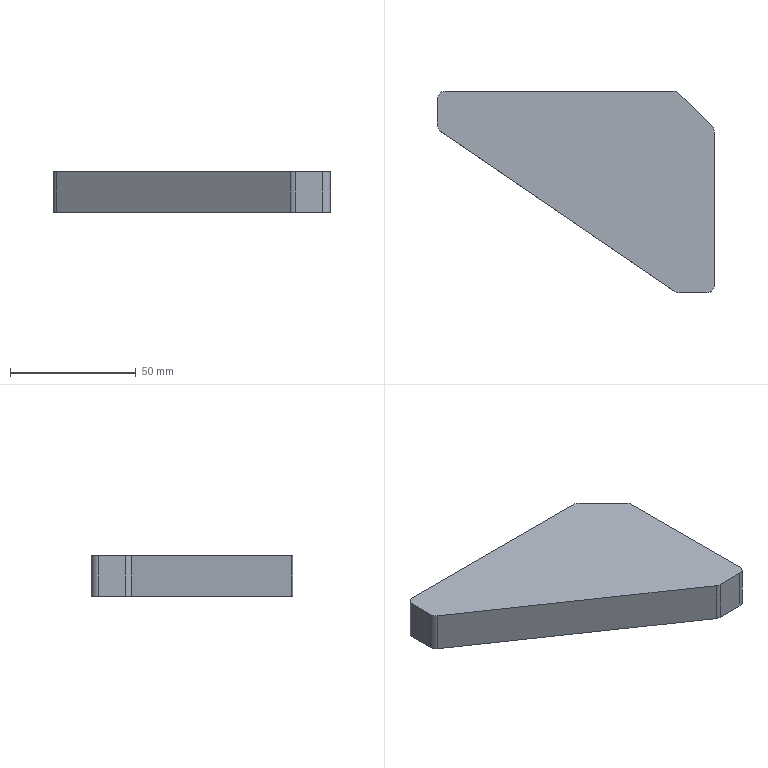Part | STEP file | Copy (1) of SN10_008_007-03_REFORCO | 1 solid | 14 faces | box 110 x 80 x 16 mm | volume 89525 mm3 | plane 8 | cylinder 6 | commonest cylinder face diameters 6 x6
STEP:
#1=CARTESIAN_POINT('',(0.,0.,0.));
#2=DIRECTION('',(0.,0.,1.));
#3=DIRECTION('',(1.,0.,0.));
#4=AXIS2_PLACEMENT_3D('',#1,#2,#3);
#5=CARTESIAN_POINT('',(243.629,237.,420.27));
#6=VERTEX_POINT('',#5);
#7=CARTESIAN_POINT('',(246.629,240.,420.27));
#8=VERTEX_POINT('',#7);
#9=CARTESIAN_POINT('',(246.629,237.,420.27));
#10=DIRECTION('',(0.,0.,-1.));
#11=DIRECTION('',(1.,0.,0.));
#12=AXIS2_PLACEMENT_3D('',#9,#10,#11);
#13=CIRCLE('',#12,3.);
#14=CARTESIAN_POINT('',(246.629,237.,428.27));
#15=DIRECTION('',(0.,0.,-1.));
#16=DIRECTION('',(-1.,0.,0.));
#17=AXIS2_PLACEMENT_3D('',#14,#15,#16);
#18=CYLINDRICAL_SURFACE('',#17,3.);
#19=CARTESIAN_POINT('',(-3.142,8.));
#20=DIRECTION('',(1.,0.));
#21=VECTOR('',#20,1.);
#22=LINE('',#19,#21);
#23=(GEOMETRIC_REPRESENTATION_CONTEXT(2)PARAMETRIC_REPRESENTATION_CONTEXT()REPRESENTATION_CONTEXT('',''));
#24=DEFINITIONAL_REPRESENTATION('',(#22),#23);
#25=PCURVE('',#18,#24);
#26=CARTESIAN_POINT('',(0.,0.,420.27));
#27=DIRECTION('',(0.,0.,-1.));
#28=DIRECTION('',(-1.,0.,0.));
#29=AXIS2_PLACEMENT_3D('',#26,#27,#28);
#30=PLANE('',#29);
#31=CARTESIAN_POINT('',(-246.629,237.));
#32=DIRECTION('',(-1.,0.));
#33=AXIS2_PLACEMENT_2D('',#31,#32);
#34=CIRCLE('',#33,3.);
#35=(GEOMETRIC_REPRESENTATION_CONTEXT(2)PARAMETRIC_REPRESENTATION_CONTEXT()REPRESENTATION_CONTEXT('',''));
#36=DEFINITIONAL_REPRESENTATION('',(#34),#35);
#37=PCURVE('',#30,#36);
#38=SURFACE_CURVE('',#13,(#25,#37),.PCURVE_S1.);
#39=EDGE_CURVE('',#6,#8,#38,.T.);
#40=ORIENTED_EDGE('',*,*,#39,.F.);
#41=CARTESIAN_POINT('',(243.629,237.,436.27));
#42=VERTEX_POINT('',#41);
#43=CARTESIAN_POINT('',(243.629,237.,436.27));
#44=DIRECTION('',(0.,0.,-1.));
#45=VECTOR('',#44,1.);
#46=LINE('',#43,#45);
#47=CARTESIAN_POINT('',(0.,-8.));
#48=DIRECTION('',(0.,1.));
#49=VECTOR('',#48,1.);
#50=LINE('',#47,#49);
#51=(GEOMETRIC_REPRESENTATION_CONTEXT(2)PARAMETRIC_REPRESENTATION_CONTEXT()REPRESENTATION_CONTEXT('',''));
#52=DEFINITIONAL_REPRESENTATION('',(#50),#51);
#53=PCURVE('',#18,#52);
#54=CARTESIAN_POINT('',(243.629,225.,436.27));
#55=DIRECTION('',(-1.,0.,0.));
#56=DIRECTION('',(0.,0.,1.));
#57=AXIS2_PLACEMENT_3D('',#54,#55,#56);
#58=PLANE('',#57);
#59=CARTESIAN_POINT('',(0.,12.));
#60=DIRECTION('',(-1.,0.));
#61=VECTOR('',#60,1.);
#62=LINE('',#59,#61);
#63=(GEOMETRIC_REPRESENTATION_CONTEXT(2)PARAMETRIC_REPRESENTATION_CONTEXT()REPRESENTATION_CONTEXT('',''));
#64=DEFINITIONAL_REPRESENTATION('',(#62),#63);
#65=PCURVE('',#58,#64);
#66=SURFACE_CURVE('',#46,(#53,#65),.PCURVE_S1.);
#67=EDGE_CURVE('',#42,#6,#66,.T.);
#68=ORIENTED_EDGE('',*,*,#67,.F.);
#69=CARTESIAN_POINT('',(246.629,240.,436.27));
#70=VERTEX_POINT('',#69);
#71=CARTESIAN_POINT('',(246.629,237.,436.27));
#72=DIRECTION('',(0.,0.,-1.));
#73=DIRECTION('',(1.,0.,0.));
#74=AXIS2_PLACEMENT_3D('',#71,#72,#73);
#75=CIRCLE('',#74,3.);
#76=CARTESIAN_POINT('',(-3.142,-8.));
#77=DIRECTION('',(1.,0.));
#78=VECTOR('',#77,1.);
#79=LINE('',#76,#78);
#80=(GEOMETRIC_REPRESENTATION_CONTEXT(2)PARAMETRIC_REPRESENTATION_CONTEXT()REPRESENTATION_CONTEXT('',''));
#81=DEFINITIONAL_REPRESENTATION('',(#79),#80);
#82=PCURVE('',#18,#81);
#83=CARTESIAN_POINT('',(0.,0.,436.27));
#84=DIRECTION('',(0.,0.,-1.));
#85=DIRECTION('',(-1.,0.,0.));
#86=AXIS2_PLACEMENT_3D('',#83,#84,#85);
#87=PLANE('',#86);
#88=CARTESIAN_POINT('',(-246.629,237.));
#89=DIRECTION('',(-1.,0.));
#90=AXIS2_PLACEMENT_2D('',#88,#89);
#91=CIRCLE('',#90,3.);
#92=(GEOMETRIC_REPRESENTATION_CONTEXT(2)PARAMETRIC_REPRESENTATION_CONTEXT()REPRESENTATION_CONTEXT('',''));
#93=DEFINITIONAL_REPRESENTATION('',(#91),#92);
#94=PCURVE('',#87,#93);
#95=SURFACE_CURVE('',#75,(#82,#94),.PCURVE_S1.);
#96=EDGE_CURVE('',#42,#70,#95,.T.);
#97=ORIENTED_EDGE('',*,*,#96,.T.);
#98=CARTESIAN_POINT('',(246.629,240.,436.27));
#99=DIRECTION('',(0.,0.,-1.));
#100=VECTOR('',#99,1.);
#101=LINE('',#98,#100);
#102=CARTESIAN_POINT('',(1.571,-8.));
#103=DIRECTION('',(0.,1.));
#104=VECTOR('',#103,1.);
#105=LINE('',#102,#104);
#106=(GEOMETRIC_REPRESENTATION_CONTEXT(2)PARAMETRIC_REPRESENTATION_CONTEXT()REPRESENTATION_CONTEXT('',''));
#107=DEFINITIONAL_REPRESENTATION('',(#105),#106);
#108=PCURVE('',#18,#107);
#109=CARTESIAN_POINT('',(243.629,240.,436.27));
#110=DIRECTION('',(0.,1.,0.));
#111=DIRECTION('',(0.,0.,1.));
#112=AXIS2_PLACEMENT_3D('',#109,#110,#111);
#113=PLANE('',#112);
#114=CARTESIAN_POINT('',(0.,3.));
#115=DIRECTION('',(-1.,0.));
#116=VECTOR('',#115,1.);
#117=LINE('',#114,#116);
#118=(GEOMETRIC_REPRESENTATION_CONTEXT(2)PARAMETRIC_REPRESENTATION_CONTEXT()REPRESENTATION_CONTEXT('',''));
#119=DEFINITIONAL_REPRESENTATION('',(#117),#118);
#120=PCURVE('',#113,#119);
#121=SURFACE_CURVE('',#101,(#108,#120),.PCURVE_S1.);
#122=EDGE_CURVE('',#70,#8,#121,.T.);
#123=ORIENTED_EDGE('',*,*,#122,.T.);
#124=EDGE_LOOP('',(#40,#68,#97,#123));
#125=FACE_BOUND('',#124,.T.);
#126=ADVANCED_FACE('',(#125),#18,.T.);
#127=CARTESIAN_POINT('',(243.629,226.582,436.27));
#128=VERTEX_POINT('',#127);
#129=CARTESIAN_POINT('',(243.629,226.582,436.27));
#130=DIRECTION('',(0.,1.,0.));
#131=VECTOR('',#130,1.);
#132=LINE('',#129,#131);
#133=CARTESIAN_POINT('',(0.,1.582));
#134=DIRECTION('',(0.,1.));
#135=VECTOR('',#134,1.);
#136=LINE('',#133,#135);
#137=(GEOMETRIC_REPRESENTATION_CONTEXT(2)PARAMETRIC_REPRESENTATION_CONTEXT()REPRESENTATION_CONTEXT('',''));
#138=DEFINITIONAL_REPRESENTATION('',(#136),#137);
#139=PCURVE('',#58,#138);
#140=CARTESIAN_POINT('',(-243.629,226.582));
#141=DIRECTION('',(0.,1.));
#142=VECTOR('',#141,1.);
#143=LINE('',#140,#142);
#144=(GEOMETRIC_REPRESENTATION_CONTEXT(2)PARAMETRIC_REPRESENTATION_CONTEXT()REPRESENTATION_CONTEXT('',''));
#145=DEFINITIONAL_REPRESENTATION('',(#143),#144);
#146=PCURVE('',#87,#145);
#147=SURFACE_CURVE('',#132,(#139,#146),.PCURVE_S1.);
#148=EDGE_CURVE('',#128,#42,#147,.T.);
#149=ORIENTED_EDGE('',*,*,#148,.T.);
#150=ORIENTED_EDGE('',*,*,#67,.T.);
#151=CARTESIAN_POINT('',(243.629,226.582,420.27));
#152=VERTEX_POINT('',#151);
#153=CARTESIAN_POINT('',(243.629,226.582,420.27));
#154=DIRECTION('',(0.,1.,0.));
#155=VECTOR('',#154,1.);
#156=LINE('',#153,#155);
#157=CARTESIAN_POINT('',(-16.,1.582));
#158=DIRECTION('',(0.,1.));
#159=VECTOR('',#158,1.);
#160=LINE('',#157,#159);
#161=(GEOMETRIC_REPRESENTATION_CONTEXT(2)PARAMETRIC_REPRESENTATION_CONTEXT()REPRESENTATION_CONTEXT('',''));
#162=DEFINITIONAL_REPRESENTATION('',(#160),#161);
#163=PCURVE('',#58,#162);
#164=CARTESIAN_POINT('',(-243.629,226.582));
#165=DIRECTION('',(0.,1.));
#166=VECTOR('',#165,1.);
#167=LINE('',#164,#166);
#168=(GEOMETRIC_REPRESENTATION_CONTEXT(2)PARAMETRIC_REPRESENTATION_CONTEXT()REPRESENTATION_CONTEXT('',''));
#169=DEFINITIONAL_REPRESENTATION('',(#167),#168);
#170=PCURVE('',#30,#169);
#171=SURFACE_CURVE('',#156,(#163,#170),.PCURVE_S1.);
#172=EDGE_CURVE('',#152,#6,#171,.T.);
#173=ORIENTED_EDGE('',*,*,#172,.F.);
#174=CARTESIAN_POINT('',(243.629,226.582,436.27));
#175=DIRECTION('',(0.,0.,-1.));
#176=VECTOR('',#175,1.);
#177=LINE('',#174,#176);
#178=CARTESIAN_POINT('',(0.,1.582));
#179=DIRECTION('',(-1.,0.));
#180=VECTOR('',#179,1.);
#181=LINE('',#178,#180);
#182=(GEOMETRIC_REPRESENTATION_CONTEXT(2)PARAMETRIC_REPRESENTATION_CONTEXT()REPRESENTATION_CONTEXT('',''));
#183=DEFINITIONAL_REPRESENTATION('',(#181),#182);
#184=PCURVE('',#58,#183);
#185=CARTESIAN_POINT('',(246.629,226.582,428.27));
#186=DIRECTION('',(0.,0.,-1.));
#187=DIRECTION('',(-0.5647,-0.8253,0.));
#188=AXIS2_PLACEMENT_3D('',#185,#186,#187);
#189=CYLINDRICAL_SURFACE('',#188,3.);
#190=CARTESIAN_POINT('',(0.9707,-8.));
#191=DIRECTION('',(0.,1.));
#192=VECTOR('',#191,1.);
#193=LINE('',#190,#192);
#194=(GEOMETRIC_REPRESENTATION_CONTEXT(2)PARAMETRIC_REPRESENTATION_CONTEXT()REPRESENTATION_CONTEXT('',''));
#195=DEFINITIONAL_REPRESENTATION('',(#193),#194);
#196=PCURVE('',#189,#195);
#197=SURFACE_CURVE('',#177,(#184,#196),.PCURVE_S1.);
#198=EDGE_CURVE('',#128,#152,#197,.T.);
#199=ORIENTED_EDGE('',*,*,#198,.F.);
#200=EDGE_LOOP('',(#149,#150,#173,#199));
#201=FACE_BOUND('',#200,.T.);
#202=ADVANCED_FACE('',(#201),#58,.T.);
#203=CARTESIAN_POINT('',(244.935,224.106,420.27));
#204=VERTEX_POINT('',#203);
#205=CARTESIAN_POINT('',(246.629,226.582,420.27));
#206=DIRECTION('',(0.,0.,-1.));
#207=DIRECTION('',(1.,0.,0.));
#208=AXIS2_PLACEMENT_3D('',#205,#206,#207);
#209=CIRCLE('',#208,3.);
#210=CARTESIAN_POINT('',(-2.171,8.));
#211=DIRECTION('',(1.,0.));
#212=VECTOR('',#211,1.);
#213=LINE('',#210,#212);
#214=(GEOMETRIC_REPRESENTATION_CONTEXT(2)PARAMETRIC_REPRESENTATION_CONTEXT()REPRESENTATION_CONTEXT('',''));
#215=DEFINITIONAL_REPRESENTATION('',(#213),#214);
#216=PCURVE('',#189,#215);
#217=CARTESIAN_POINT('',(-246.629,226.582));
#218=DIRECTION('',(-1.,0.));
#219=AXIS2_PLACEMENT_2D('',#217,#218);
#220=CIRCLE('',#219,3.);
#221=(GEOMETRIC_REPRESENTATION_CONTEXT(2)PARAMETRIC_REPRESENTATION_CONTEXT()REPRESENTATION_CONTEXT('',''));
#222=DEFINITIONAL_REPRESENTATION('',(#220),#221);
#223=PCURVE('',#30,#222);
#224=SURFACE_CURVE('',#209,(#216,#223),.PCURVE_S1.);
#225=EDGE_CURVE('',#204,#152,#224,.T.);
#226=ORIENTED_EDGE('',*,*,#225,.F.);
#227=CARTESIAN_POINT('',(244.935,224.106,436.27));
#228=VERTEX_POINT('',#227);
#229=CARTESIAN_POINT('',(244.935,224.106,436.27));
#230=DIRECTION('',(0.,0.,-1.));
#231=VECTOR('',#230,1.);
#232=LINE('',#229,#231);
#233=CARTESIAN_POINT('',(0.,-8.));
#234=DIRECTION('',(0.,1.));
#235=VECTOR('',#234,1.);
#236=LINE('',#233,#235);
#237=(GEOMETRIC_REPRESENTATION_CONTEXT(2)PARAMETRIC_REPRESENTATION_CONTEXT()REPRESENTATION_CONTEXT('',''));
#238=DEFINITIONAL_REPRESENTATION('',(#236),#237);
#239=PCURVE('',#189,#238);
#240=CARTESIAN_POINT('',(338.629,160.,436.27));
#241=DIRECTION('',(-0.5647,-0.8253,0.));
#242=DIRECTION('',(0.,0.,1.));
#243=AXIS2_PLACEMENT_3D('',#240,#241,#242);
#244=PLANE('',#243);
#245=CARTESIAN_POINT('',(0.,113.526));
#246=DIRECTION('',(-1.,0.));
#247=VECTOR('',#246,1.);
#248=LINE('',#245,#247);
#249=(GEOMETRIC_REPRESENTATION_CONTEXT(2)PARAMETRIC_REPRESENTATION_CONTEXT()REPRESENTATION_CONTEXT('',''));
#250=DEFINITIONAL_REPRESENTATION('',(#248),#249);
#251=PCURVE('',#244,#250);
#252=SURFACE_CURVE('',#232,(#239,#251),.PCURVE_S1.);
#253=EDGE_CURVE('',#228,#204,#252,.T.);
#254=ORIENTED_EDGE('',*,*,#253,.F.);
#255=CARTESIAN_POINT('',(246.629,226.582,436.27));
#256=DIRECTION('',(0.,0.,-1.));
#257=DIRECTION('',(1.,0.,0.));
#258=AXIS2_PLACEMENT_3D('',#255,#256,#257);
#259=CIRCLE('',#258,3.);
#260=CARTESIAN_POINT('',(-2.171,-8.));
#261=DIRECTION('',(1.,0.));
#262=VECTOR('',#261,1.);
#263=LINE('',#260,#262);
#264=(GEOMETRIC_REPRESENTATION_CONTEXT(2)PARAMETRIC_REPRESENTATION_CONTEXT()REPRESENTATION_CONTEXT('',''));
#265=DEFINITIONAL_REPRESENTATION('',(#263),#264);
#266=PCURVE('',#189,#265);
#267=CARTESIAN_POINT('',(-246.629,226.582));
#268=DIRECTION('',(-1.,0.));
#269=AXIS2_PLACEMENT_2D('',#267,#268);
#270=CIRCLE('',#269,3.);
#271=(GEOMETRIC_REPRESENTATION_CONTEXT(2)PARAMETRIC_REPRESENTATION_CONTEXT()REPRESENTATION_CONTEXT('',''));
#272=DEFINITIONAL_REPRESENTATION('',(#270),#271);
#273=PCURVE('',#87,#272);
#274=SURFACE_CURVE('',#259,(#266,#273),.PCURVE_S1.);
#275=EDGE_CURVE('',#228,#128,#274,.T.);
#276=ORIENTED_EDGE('',*,*,#275,.T.);
#277=ORIENTED_EDGE('',*,*,#198,.T.);
#278=EDGE_LOOP('',(#226,#254,#276,#277));
#279=FACE_BOUND('',#278,.T.);
#280=ADVANCED_FACE('',(#279),#189,.T.);
#281=CARTESIAN_POINT('',(337.863,160.524,436.27));
#282=VERTEX_POINT('',#281);
#283=CARTESIAN_POINT('',(337.863,160.524,436.27));
#284=DIRECTION('',(-0.8253,0.5647,0.));
#285=VECTOR('',#284,1.);
#286=LINE('',#283,#285);
#287=CARTESIAN_POINT('',(0.,0.9281));
#288=DIRECTION('',(0.,1.));
#289=VECTOR('',#288,1.);
#290=LINE('',#287,#289);
#291=(GEOMETRIC_REPRESENTATION_CONTEXT(2)PARAMETRIC_REPRESENTATION_CONTEXT()REPRESENTATION_CONTEXT('',''));
#292=DEFINITIONAL_REPRESENTATION('',(#290),#291);
#293=PCURVE('',#244,#292);
#294=CARTESIAN_POINT('',(-337.863,160.524));
#295=DIRECTION('',(0.8253,0.5647));
#296=VECTOR('',#295,1.);
#297=LINE('',#294,#296);
#298=(GEOMETRIC_REPRESENTATION_CONTEXT(2)PARAMETRIC_REPRESENTATION_CONTEXT()REPRESENTATION_CONTEXT('',''));
#299=DEFINITIONAL_REPRESENTATION('',(#297),#298);
#300=PCURVE('',#87,#299);
#301=SURFACE_CURVE('',#286,(#293,#300),.PCURVE_S1.);
#302=EDGE_CURVE('',#282,#228,#301,.T.);
#303=ORIENTED_EDGE('',*,*,#302,.T.);
#304=ORIENTED_EDGE('',*,*,#253,.T.);
#305=CARTESIAN_POINT('',(337.863,160.524,420.27));
#306=VERTEX_POINT('',#305);
#307=CARTESIAN_POINT('',(337.863,160.524,420.27));
#308=DIRECTION('',(-0.8253,0.5647,0.));
#309=VECTOR('',#308,1.);
#310=LINE('',#307,#309);
#311=CARTESIAN_POINT('',(-16.,0.9281));
#312=DIRECTION('',(0.,1.));
#313=VECTOR('',#312,1.);
#314=LINE('',#311,#313);
#315=(GEOMETRIC_REPRESENTATION_CONTEXT(2)PARAMETRIC_REPRESENTATION_CONTEXT()REPRESENTATION_CONTEXT('',''));
#316=DEFINITIONAL_REPRESENTATION('',(#314),#315);
#317=PCURVE('',#244,#316);
#318=CARTESIAN_POINT('',(-337.863,160.524));
#319=DIRECTION('',(0.8253,0.5647));
#320=VECTOR('',#319,1.);
#321=LINE('',#318,#320);
#322=(GEOMETRIC_REPRESENTATION_CONTEXT(2)PARAMETRIC_REPRESENTATION_CONTEXT()REPRESENTATION_CONTEXT('',''));
#323=DEFINITIONAL_REPRESENTATION('',(#321),#322);
#324=PCURVE('',#30,#323);
#325=SURFACE_CURVE('',#310,(#317,#324),.PCURVE_S1.);
#326=EDGE_CURVE('',#306,#204,#325,.T.);
#327=ORIENTED_EDGE('',*,*,#326,.F.);
#328=CARTESIAN_POINT('',(337.863,160.524,436.27));
#329=DIRECTION('',(0.,0.,-1.));
#330=VECTOR('',#329,1.);
#331=LINE('',#328,#330);
#332=CARTESIAN_POINT('',(0.,0.9281));
#333=DIRECTION('',(-1.,0.));
#334=VECTOR('',#333,1.);
#335=LINE('',#332,#334);
#336=(GEOMETRIC_REPRESENTATION_CONTEXT(2)PARAMETRIC_REPRESENTATION_CONTEXT()REPRESENTATION_CONTEXT('',''));
#337=DEFINITIONAL_REPRESENTATION('',(#335),#336);
#338=PCURVE('',#244,#337);
#339=CARTESIAN_POINT('',(339.557,163.,428.27));
#340=DIRECTION('',(0.,0.,-1.));
#341=DIRECTION('',(0.,-1.,0.));
#342=AXIS2_PLACEMENT_3D('',#339,#340,#341);
#343=CYLINDRICAL_SURFACE('',#342,3.);
#344=CARTESIAN_POINT('',(0.6001,-8.));
#345=DIRECTION('',(0.,1.));
#346=VECTOR('',#345,1.);
#347=LINE('',#344,#346);
#348=(GEOMETRIC_REPRESENTATION_CONTEXT(2)PARAMETRIC_REPRESENTATION_CONTEXT()REPRESENTATION_CONTEXT('',''));
#349=DEFINITIONAL_REPRESENTATION('',(#347),#348);
#350=PCURVE('',#343,#349);
#351=SURFACE_CURVE('',#331,(#338,#350),.PCURVE_S1.);
#352=EDGE_CURVE('',#282,#306,#351,.T.);
#353=ORIENTED_EDGE('',*,*,#352,.F.);
#354=EDGE_LOOP('',(#303,#304,#327,#353));
#355=FACE_BOUND('',#354,.T.);
#356=ADVANCED_FACE('',(#355),#244,.T.);
#357=CARTESIAN_POINT('',(339.557,160.,420.27));
#358=VERTEX_POINT('',#357);
#359=CARTESIAN_POINT('',(339.557,163.,420.27));
#360=DIRECTION('',(0.,0.,-1.));
#361=DIRECTION('',(1.,0.,0.));
#362=AXIS2_PLACEMENT_3D('',#359,#360,#361);
#363=CIRCLE('',#362,3.);
#364=CARTESIAN_POINT('',(-1.571,8.));
#365=DIRECTION('',(1.,0.));
#366=VECTOR('',#365,1.);
#367=LINE('',#364,#366);
#368=(GEOMETRIC_REPRESENTATION_CONTEXT(2)PARAMETRIC_REPRESENTATION_CONTEXT()REPRESENTATION_CONTEXT('',''));
#369=DEFINITIONAL_REPRESENTATION('',(#367),#368);
#370=PCURVE('',#343,#369);
#371=CARTESIAN_POINT('',(-339.557,163.));
#372=DIRECTION('',(-1.,0.));
#373=AXIS2_PLACEMENT_2D('',#371,#372);
#374=CIRCLE('',#373,3.);
#375=(GEOMETRIC_REPRESENTATION_CONTEXT(2)PARAMETRIC_REPRESENTATION_CONTEXT()REPRESENTATION_CONTEXT('',''));
#376=DEFINITIONAL_REPRESENTATION('',(#374),#375);
#377=PCURVE('',#30,#376);
#378=SURFACE_CURVE('',#363,(#370,#377),.PCURVE_S1.);
#379=EDGE_CURVE('',#358,#306,#378,.T.);
#380=ORIENTED_EDGE('',*,*,#379,.F.);
#381=CARTESIAN_POINT('',(339.557,160.,436.27));
#382=VERTEX_POINT('',#381);
#383=CARTESIAN_POINT('',(339.557,160.,436.27));
#384=DIRECTION('',(0.,0.,-1.));
#385=VECTOR('',#384,1.);
#386=LINE('',#383,#385);
#387=CARTESIAN_POINT('',(0.,-8.));
#388=DIRECTION('',(0.,1.));
#389=VECTOR('',#388,1.);
#390=LINE('',#387,#389);
#391=(GEOMETRIC_REPRESENTATION_CONTEXT(2)PARAMETRIC_REPRESENTATION_CONTEXT()REPRESENTATION_CONTEXT('',''));
#392=DEFINITIONAL_REPRESENTATION('',(#390),#391);
#393=PCURVE('',#343,#392);
#394=CARTESIAN_POINT('',(353.629,160.,436.27));
#395=DIRECTION('',(0.,-1.,0.));
#396=DIRECTION('',(0.,0.,-1.));
#397=AXIS2_PLACEMENT_3D('',#394,#395,#396);
#398=PLANE('',#397);
#399=CARTESIAN_POINT('',(0.,-14.072));
#400=DIRECTION('',(1.,0.));
#401=VECTOR('',#400,1.);
#402=LINE('',#399,#401);
#403=(GEOMETRIC_REPRESENTATION_CONTEXT(2)PARAMETRIC_REPRESENTATION_CONTEXT()REPRESENTATION_CONTEXT('',''));
#404=DEFINITIONAL_REPRESENTATION('',(#402),#403);
#405=PCURVE('',#398,#404);
#406=SURFACE_CURVE('',#386,(#393,#405),.PCURVE_S1.);
#407=EDGE_CURVE('',#382,#358,#406,.T.);
#408=ORIENTED_EDGE('',*,*,#407,.F.);
#409=CARTESIAN_POINT('',(339.557,163.,436.27));
#410=DIRECTION('',(0.,0.,-1.));
#411=DIRECTION('',(1.,0.,0.));
#412=AXIS2_PLACEMENT_3D('',#409,#410,#411);
#413=CIRCLE('',#412,3.);
#414=CARTESIAN_POINT('',(-1.571,-8.));
#415=DIRECTION('',(1.,0.));
#416=VECTOR('',#415,1.);
#417=LINE('',#414,#416);
#418=(GEOMETRIC_REPRESENTATION_CONTEXT(2)PARAMETRIC_REPRESENTATION_CONTEXT()REPRESENTATION_CONTEXT('',''));
#419=DEFINITIONAL_REPRESENTATION('',(#417),#418);
#420=PCURVE('',#343,#419);
#421=CARTESIAN_POINT('',(-339.557,163.));
#422=DIRECTION('',(-1.,0.));
#423=AXIS2_PLACEMENT_2D('',#421,#422);
#424=CIRCLE('',#423,3.);
#425=(GEOMETRIC_REPRESENTATION_CONTEXT(2)PARAMETRIC_REPRESENTATION_CONTEXT()REPRESENTATION_CONTEXT('',''));
#426=DEFINITIONAL_REPRESENTATION('',(#424),#425);
#427=PCURVE('',#87,#426);
#428=SURFACE_CURVE('',#413,(#420,#427),.PCURVE_S1.);
#429=EDGE_CURVE('',#382,#282,#428,.T.);
#430=ORIENTED_EDGE('',*,*,#429,.T.);
#431=ORIENTED_EDGE('',*,*,#352,.T.);
#432=EDGE_LOOP('',(#380,#408,#430,#431));
#433=FACE_BOUND('',#432,.T.);
#434=ADVANCED_FACE('',(#433),#343,.T.);
#435=CARTESIAN_POINT('',(350.629,160.,436.27));
#436=VERTEX_POINT('',#435);
#437=CARTESIAN_POINT('',(350.629,160.,436.27));
#438=DIRECTION('',(-1.,0.,0.));
#439=VECTOR('',#438,1.);
#440=LINE('',#437,#439);
#441=CARTESIAN_POINT('',(0.,-3.));
#442=DIRECTION('',(0.,-1.));
#443=VECTOR('',#442,1.);
#444=LINE('',#441,#443);
#445=(GEOMETRIC_REPRESENTATION_CONTEXT(2)PARAMETRIC_REPRESENTATION_CONTEXT()REPRESENTATION_CONTEXT('',''));
#446=DEFINITIONAL_REPRESENTATION('',(#444),#445);
#447=PCURVE('',#398,#446);
#448=CARTESIAN_POINT('',(-350.629,160.));
#449=DIRECTION('',(1.,0.));
#450=VECTOR('',#449,1.);
#451=LINE('',#448,#450);
#452=(GEOMETRIC_REPRESENTATION_CONTEXT(2)PARAMETRIC_REPRESENTATION_CONTEXT()REPRESENTATION_CONTEXT('',''));
#453=DEFINITIONAL_REPRESENTATION('',(#451),#452);
#454=PCURVE('',#87,#453);
#455=SURFACE_CURVE('',#440,(#447,#454),.PCURVE_S1.);
#456=EDGE_CURVE('',#436,#382,#455,.T.);
#457=ORIENTED_EDGE('',*,*,#456,.T.);
#458=ORIENTED_EDGE('',*,*,#407,.T.);
#459=CARTESIAN_POINT('',(350.629,160.,420.27));
#460=VERTEX_POINT('',#459);
#461=CARTESIAN_POINT('',(350.629,160.,420.27));
#462=DIRECTION('',(-1.,0.,0.));
#463=VECTOR('',#462,1.);
#464=LINE('',#461,#463);
#465=CARTESIAN_POINT('',(16.,-3.));
#466=DIRECTION('',(0.,-1.));
#467=VECTOR('',#466,1.);
#468=LINE('',#465,#467);
#469=(GEOMETRIC_REPRESENTATION_CONTEXT(2)PARAMETRIC_REPRESENTATION_CONTEXT()REPRESENTATION_CONTEXT('',''));
#470=DEFINITIONAL_REPRESENTATION('',(#468),#469);
#471=PCURVE('',#398,#470);
#472=CARTESIAN_POINT('',(-350.629,160.));
#473=DIRECTION('',(1.,0.));
#474=VECTOR('',#473,1.);
#475=LINE('',#472,#474);
#476=(GEOMETRIC_REPRESENTATION_CONTEXT(2)PARAMETRIC_REPRESENTATION_CONTEXT()REPRESENTATION_CONTEXT('',''));
#477=DEFINITIONAL_REPRESENTATION('',(#475),#476);
#478=PCURVE('',#30,#477);
#479=SURFACE_CURVE('',#464,(#471,#478),.PCURVE_S1.);
#480=EDGE_CURVE('',#460,#358,#479,.T.);
#481=ORIENTED_EDGE('',*,*,#480,.F.);
#482=CARTESIAN_POINT('',(350.629,160.,436.27));
#483=DIRECTION('',(0.,0.,-1.));
#484=VECTOR('',#483,1.);
#485=LINE('',#482,#484);
#486=CARTESIAN_POINT('',(0.,-3.));
#487=DIRECTION('',(1.,0.));
#488=VECTOR('',#487,1.);
#489=LINE('',#486,#488);
#490=(GEOMETRIC_REPRESENTATION_CONTEXT(2)PARAMETRIC_REPRESENTATION_CONTEXT()REPRESENTATION_CONTEXT('',''));
#491=DEFINITIONAL_REPRESENTATION('',(#489),#490);
#492=PCURVE('',#398,#491);
#493=CARTESIAN_POINT('',(350.629,163.,428.27));
#494=DIRECTION('',(0.,0.,-1.));
#495=DIRECTION('',(1.,0.,0.));
#496=AXIS2_PLACEMENT_3D('',#493,#494,#495);
#497=CYLINDRICAL_SURFACE('',#496,3.);
#498=CARTESIAN_POINT('',(1.571,-8.));
#499=DIRECTION('',(0.,1.));
#500=VECTOR('',#499,1.);
#501=LINE('',#498,#500);
#502=(GEOMETRIC_REPRESENTATION_CONTEXT(2)PARAMETRIC_REPRESENTATION_CONTEXT()REPRESENTATION_CONTEXT('',''));
#503=DEFINITIONAL_REPRESENTATION('',(#501),#502);
#504=PCURVE('',#497,#503);
#505=SURFACE_CURVE('',#485,(#492,#504),.PCURVE_S1.);
#506=EDGE_CURVE('',#436,#460,#505,.T.);
#507=ORIENTED_EDGE('',*,*,#506,.F.);
#508=EDGE_LOOP('',(#457,#458,#481,#507));
#509=FACE_BOUND('',#508,.T.);
#510=ADVANCED_FACE('',(#509),#398,.T.);
#511=CARTESIAN_POINT('',(353.629,163.,420.27));
#512=VERTEX_POINT('',#511);
#513=CARTESIAN_POINT('',(350.629,163.,420.27));
#514=DIRECTION('',(0.,0.,-1.));
#515=DIRECTION('',(1.,0.,0.));
#516=AXIS2_PLACEMENT_3D('',#513,#514,#515);
#517=CIRCLE('',#516,3.);
#518=CARTESIAN_POINT('',(0.,8.));
#519=DIRECTION('',(1.,0.));
#520=VECTOR('',#519,1.);
#521=LINE('',#518,#520);
#522=(GEOMETRIC_REPRESENTATION_CONTEXT(2)PARAMETRIC_REPRESENTATION_CONTEXT()REPRESENTATION_CONTEXT('',''));
#523=DEFINITIONAL_REPRESENTATION('',(#521),#522);
#524=PCURVE('',#497,#523);
#525=CARTESIAN_POINT('',(-350.629,163.));
#526=DIRECTION('',(-1.,0.));
#527=AXIS2_PLACEMENT_2D('',#525,#526);
#528=CIRCLE('',#527,3.);
#529=(GEOMETRIC_REPRESENTATION_CONTEXT(2)PARAMETRIC_REPRESENTATION_CONTEXT()REPRESENTATION_CONTEXT('',''));
#530=DEFINITIONAL_REPRESENTATION('',(#528),#529);
#531=PCURVE('',#30,#530);
#532=SURFACE_CURVE('',#517,(#524,#531),.PCURVE_S1.);
#533=EDGE_CURVE('',#512,#460,#532,.T.);
#534=ORIENTED_EDGE('',*,*,#533,.F.);
#535=CARTESIAN_POINT('',(353.629,163.,436.27));
#536=VERTEX_POINT('',#535);
#537=CARTESIAN_POINT('',(353.629,163.,436.27));
#538=DIRECTION('',(0.,0.,-1.));
#539=VECTOR('',#538,1.);
#540=LINE('',#537,#539);
#541=CARTESIAN_POINT('',(0.,-8.));
#542=DIRECTION('',(0.,1.));
#543=VECTOR('',#542,1.);
#544=LINE('',#541,#543);
#545=(GEOMETRIC_REPRESENTATION_CONTEXT(2)PARAMETRIC_REPRESENTATION_CONTEXT()REPRESENTATION_CONTEXT('',''));
#546=DEFINITIONAL_REPRESENTATION('',(#544),#545);
#547=PCURVE('',#497,#546);
#548=CARTESIAN_POINT('',(353.629,225.,436.27));
#549=DIRECTION('',(1.,0.,0.));
#550=DIRECTION('',(0.,0.,-1.));
#551=AXIS2_PLACEMENT_3D('',#548,#549,#550);
#552=PLANE('',#551);
#553=CARTESIAN_POINT('',(0.,-62.));
#554=DIRECTION('',(1.,0.));
#555=VECTOR('',#554,1.);
#556=LINE('',#553,#555);
#557=(GEOMETRIC_REPRESENTATION_CONTEXT(2)PARAMETRIC_REPRESENTATION_CONTEXT()REPRESENTATION_CONTEXT('',''));
#558=DEFINITIONAL_REPRESENTATION('',(#556),#557);
#559=PCURVE('',#552,#558);
#560=SURFACE_CURVE('',#540,(#547,#559),.PCURVE_S1.);
#561=EDGE_CURVE('',#536,#512,#560,.T.);
#562=ORIENTED_EDGE('',*,*,#561,.F.);
#563=CARTESIAN_POINT('',(350.629,163.,436.27));
#564=DIRECTION('',(0.,0.,-1.));
#565=DIRECTION('',(1.,0.,0.));
#566=AXIS2_PLACEMENT_3D('',#563,#564,#565);
#567=CIRCLE('',#566,3.);
#568=CARTESIAN_POINT('',(0.,-8.));
#569=DIRECTION('',(1.,0.));
#570=VECTOR('',#569,1.);
#571=LINE('',#568,#570);
#572=(GEOMETRIC_REPRESENTATION_CONTEXT(2)PARAMETRIC_REPRESENTATION_CONTEXT()REPRESENTATION_CONTEXT('',''));
#573=DEFINITIONAL_REPRESENTATION('',(#571),#572);
#574=PCURVE('',#497,#573);
#575=CARTESIAN_POINT('',(-350.629,163.));
#576=DIRECTION('',(-1.,0.));
#577=AXIS2_PLACEMENT_2D('',#575,#576);
#578=CIRCLE('',#577,3.);
#579=(GEOMETRIC_REPRESENTATION_CONTEXT(2)PARAMETRIC_REPRESENTATION_CONTEXT()REPRESENTATION_CONTEXT('',''));
#580=DEFINITIONAL_REPRESENTATION('',(#578),#579);
#581=PCURVE('',#87,#580);
#582=SURFACE_CURVE('',#567,(#574,#581),.PCURVE_S1.);
#583=EDGE_CURVE('',#536,#436,#582,.T.);
#584=ORIENTED_EDGE('',*,*,#583,.T.);
#585=ORIENTED_EDGE('',*,*,#506,.T.);
#586=EDGE_LOOP('',(#534,#562,#584,#585));
#587=FACE_BOUND('',#586,.T.);
#588=ADVANCED_FACE('',(#587),#497,.T.);
#589=CARTESIAN_POINT('',(353.629,223.757,436.27));
#590=VERTEX_POINT('',#589);
#591=CARTESIAN_POINT('',(353.629,223.757,436.27));
#592=DIRECTION('',(0.,-1.,0.));
#593=VECTOR('',#592,1.);
#594=LINE('',#591,#593);
#595=CARTESIAN_POINT('',(0.,-1.243));
#596=DIRECTION('',(0.,-1.));
#597=VECTOR('',#596,1.);
#598=LINE('',#595,#597);
#599=(GEOMETRIC_REPRESENTATION_CONTEXT(2)PARAMETRIC_REPRESENTATION_CONTEXT()REPRESENTATION_CONTEXT('',''));
#600=DEFINITIONAL_REPRESENTATION('',(#598),#599);
#601=PCURVE('',#552,#600);
#602=CARTESIAN_POINT('',(-353.629,223.757));
#603=DIRECTION('',(0.,-1.));
#604=VECTOR('',#603,1.);
#605=LINE('',#602,#604);
#606=(GEOMETRIC_REPRESENTATION_CONTEXT(2)PARAMETRIC_REPRESENTATION_CONTEXT()REPRESENTATION_CONTEXT('',''));
#607=DEFINITIONAL_REPRESENTATION('',(#605),#606);
#608=PCURVE('',#87,#607);
#609=SURFACE_CURVE('',#594,(#601,#608),.PCURVE_S1.);
#610=EDGE_CURVE('',#590,#536,#609,.T.);
#611=ORIENTED_EDGE('',*,*,#610,.T.);
#612=ORIENTED_EDGE('',*,*,#561,.T.);
#613=CARTESIAN_POINT('',(353.629,223.757,420.27));
#614=VERTEX_POINT('',#613);
#615=CARTESIAN_POINT('',(353.629,223.757,420.27));
#616=DIRECTION('',(0.,-1.,0.));
#617=VECTOR('',#616,1.);
#618=LINE('',#615,#617);
#619=CARTESIAN_POINT('',(16.,-1.243));
#620=DIRECTION('',(0.,-1.));
#621=VECTOR('',#620,1.);
#622=LINE('',#619,#621);
#623=(GEOMETRIC_REPRESENTATION_CONTEXT(2)PARAMETRIC_REPRESENTATION_CONTEXT()REPRESENTATION_CONTEXT('',''));
#624=DEFINITIONAL_REPRESENTATION('',(#622),#623);
#625=PCURVE('',#552,#624);
#626=CARTESIAN_POINT('',(-353.629,223.757));
#627=DIRECTION('',(0.,-1.));
#628=VECTOR('',#627,1.);
#629=LINE('',#626,#628);
#630=(GEOMETRIC_REPRESENTATION_CONTEXT(2)PARAMETRIC_REPRESENTATION_CONTEXT()REPRESENTATION_CONTEXT('',''));
#631=DEFINITIONAL_REPRESENTATION('',(#629),#630);
#632=PCURVE('',#30,#631);
#633=SURFACE_CURVE('',#618,(#625,#632),.PCURVE_S1.);
#634=EDGE_CURVE('',#614,#512,#633,.T.);
#635=ORIENTED_EDGE('',*,*,#634,.F.);
#636=CARTESIAN_POINT('',(353.629,223.757,436.27));
#637=DIRECTION('',(0.,0.,-1.));
#638=VECTOR('',#637,1.);
#639=LINE('',#636,#638);
#640=CARTESIAN_POINT('',(0.,-1.243));
#641=DIRECTION('',(1.,0.));
#642=VECTOR('',#641,1.);
#643=LINE('',#640,#642);
#644=(GEOMETRIC_REPRESENTATION_CONTEXT(2)PARAMETRIC_REPRESENTATION_CONTEXT()REPRESENTATION_CONTEXT('',''));
#645=DEFINITIONAL_REPRESENTATION('',(#643),#644);
#646=PCURVE('',#552,#645);
#647=CARTESIAN_POINT('',(350.629,223.757,428.27));
#648=DIRECTION('',(0.,0.,-1.));
#649=DIRECTION('',(0.7071,0.7071,0.));
#650=AXIS2_PLACEMENT_3D('',#647,#648,#649);
#651=CYLINDRICAL_SURFACE('',#650,3.);
#652=CARTESIAN_POINT('',(0.7854,-8.));
#653=DIRECTION('',(0.,1.));
#654=VECTOR('',#653,1.);
#655=LINE('',#652,#654);
#656=(GEOMETRIC_REPRESENTATION_CONTEXT(2)PARAMETRIC_REPRESENTATION_CONTEXT()REPRESENTATION_CONTEXT('',''));
#657=DEFINITIONAL_REPRESENTATION('',(#655),#656);
#658=PCURVE('',#651,#657);
#659=SURFACE_CURVE('',#639,(#646,#658),.PCURVE_S1.);
#660=EDGE_CURVE('',#590,#614,#659,.T.);
#661=ORIENTED_EDGE('',*,*,#660,.F.);
#662=EDGE_LOOP('',(#611,#612,#635,#661));
#663=FACE_BOUND('',#662,.T.);
#664=ADVANCED_FACE('',(#663),#552,.T.);
#665=CARTESIAN_POINT('',(352.75,225.879,420.27));
#666=VERTEX_POINT('',#665);
#667=CARTESIAN_POINT('',(350.629,223.757,420.27));
#668=DIRECTION('',(0.,0.,-1.));
#669=DIRECTION('',(1.,0.,0.));
#670=AXIS2_PLACEMENT_3D('',#667,#668,#669);
#671=CIRCLE('',#670,3.);
#672=CARTESIAN_POINT('',(-5.498,8.));
#673=DIRECTION('',(1.,0.));
#674=VECTOR('',#673,1.);
#675=LINE('',#672,#674);
#676=(GEOMETRIC_REPRESENTATION_CONTEXT(2)PARAMETRIC_REPRESENTATION_CONTEXT()REPRESENTATION_CONTEXT('',''));
#677=DEFINITIONAL_REPRESENTATION('',(#675),#676);
#678=PCURVE('',#651,#677);
#679=CARTESIAN_POINT('',(-350.629,223.757));
#680=DIRECTION('',(-1.,0.));
#681=AXIS2_PLACEMENT_2D('',#679,#680);
#682=CIRCLE('',#681,3.);
#683=(GEOMETRIC_REPRESENTATION_CONTEXT(2)PARAMETRIC_REPRESENTATION_CONTEXT()REPRESENTATION_CONTEXT('',''));
#684=DEFINITIONAL_REPRESENTATION('',(#682),#683);
#685=PCURVE('',#30,#684);
#686=SURFACE_CURVE('',#671,(#678,#685),.PCURVE_S1.);
#687=EDGE_CURVE('',#666,#614,#686,.T.);
#688=ORIENTED_EDGE('',*,*,#687,.F.);
#689=CARTESIAN_POINT('',(352.75,225.879,436.27));
#690=VERTEX_POINT('',#689);
#691=CARTESIAN_POINT('',(352.75,225.879,436.27));
#692=DIRECTION('',(0.,0.,-1.));
#693=VECTOR('',#692,1.);
#694=LINE('',#691,#693);
#695=CARTESIAN_POINT('',(0.,-8.));
#696=DIRECTION('',(0.,1.));
#697=VECTOR('',#696,1.);
#698=LINE('',#695,#697);
#699=(GEOMETRIC_REPRESENTATION_CONTEXT(2)PARAMETRIC_REPRESENTATION_CONTEXT()REPRESENTATION_CONTEXT('',''));
#700=DEFINITIONAL_REPRESENTATION('',(#698),#699);
#701=PCURVE('',#651,#700);
#702=CARTESIAN_POINT('',(338.629,240.,436.27));
#703=DIRECTION('',(0.7071,0.7071,0.));
#704=DIRECTION('',(0.,0.,-1.));
#705=AXIS2_PLACEMENT_3D('',#702,#703,#704);
#706=PLANE('',#705);
#707=CARTESIAN_POINT('',(0.,-19.971));
#708=DIRECTION('',(1.,0.));
#709=VECTOR('',#708,1.);
#710=LINE('',#707,#709);
#711=(GEOMETRIC_REPRESENTATION_CONTEXT(2)PARAMETRIC_REPRESENTATION_CONTEXT()REPRESENTATION_CONTEXT('',''));
#712=DEFINITIONAL_REPRESENTATION('',(#710),#711);
#713=PCURVE('',#706,#712);
#714=SURFACE_CURVE('',#694,(#701,#713),.PCURVE_S1.);
#715=EDGE_CURVE('',#690,#666,#714,.T.);
#716=ORIENTED_EDGE('',*,*,#715,.F.);
#717=CARTESIAN_POINT('',(350.629,223.757,436.27));
#718=DIRECTION('',(0.,0.,-1.));
#719=DIRECTION('',(1.,0.,0.));
#720=AXIS2_PLACEMENT_3D('',#717,#718,#719);
#721=CIRCLE('',#720,3.);
#722=CARTESIAN_POINT('',(-5.498,-8.));
#723=DIRECTION('',(1.,0.));
#724=VECTOR('',#723,1.);
#725=LINE('',#722,#724);
#726=(GEOMETRIC_REPRESENTATION_CONTEXT(2)PARAMETRIC_REPRESENTATION_CONTEXT()REPRESENTATION_CONTEXT('',''));
#727=DEFINITIONAL_REPRESENTATION('',(#725),#726);
#728=PCURVE('',#651,#727);
#729=CARTESIAN_POINT('',(-350.629,223.757));
#730=DIRECTION('',(-1.,0.));
#731=AXIS2_PLACEMENT_2D('',#729,#730);
#732=CIRCLE('',#731,3.);
#733=(GEOMETRIC_REPRESENTATION_CONTEXT(2)PARAMETRIC_REPRESENTATION_CONTEXT()REPRESENTATION_CONTEXT('',''));
#734=DEFINITIONAL_REPRESENTATION('',(#732),#733);
#735=PCURVE('',#87,#734);
#736=SURFACE_CURVE('',#721,(#728,#735),.PCURVE_S1.);
#737=EDGE_CURVE('',#690,#590,#736,.T.);
#738=ORIENTED_EDGE('',*,*,#737,.T.);
#739=ORIENTED_EDGE('',*,*,#660,.T.);
#740=EDGE_LOOP('',(#688,#716,#738,#739));
#741=FACE_BOUND('',#740,.T.);
#742=ADVANCED_FACE('',(#741),#651,.T.);
#743=CARTESIAN_POINT('',(337.386,240.,420.27));
#744=VERTEX_POINT('',#743);
#745=CARTESIAN_POINT('',(246.629,240.,420.27));
#746=DIRECTION('',(1.,0.,0.));
#747=VECTOR('',#746,1.);
#748=LINE('',#745,#747);
#749=CARTESIAN_POINT('',(-16.,3.));
#750=DIRECTION('',(0.,1.));
#751=VECTOR('',#750,1.);
#752=LINE('',#749,#751);
#753=(GEOMETRIC_REPRESENTATION_CONTEXT(2)PARAMETRIC_REPRESENTATION_CONTEXT()REPRESENTATION_CONTEXT('',''));
#754=DEFINITIONAL_REPRESENTATION('',(#752),#753);
#755=PCURVE('',#113,#754);
#756=CARTESIAN_POINT('',(-246.629,240.));
#757=DIRECTION('',(-1.,0.));
#758=VECTOR('',#757,1.);
#759=LINE('',#756,#758);
#760=(GEOMETRIC_REPRESENTATION_CONTEXT(2)PARAMETRIC_REPRESENTATION_CONTEXT()REPRESENTATION_CONTEXT('',''));
#761=DEFINITIONAL_REPRESENTATION('',(#759),#760);
#762=PCURVE('',#30,#761);
#763=SURFACE_CURVE('',#748,(#755,#762),.PCURVE_S1.);
#764=EDGE_CURVE('',#8,#744,#763,.T.);
#765=ORIENTED_EDGE('',*,*,#764,.F.);
#766=ORIENTED_EDGE('',*,*,#122,.F.);
#767=CARTESIAN_POINT('',(337.386,240.,436.27));
#768=VERTEX_POINT('',#767);
#769=CARTESIAN_POINT('',(246.629,240.,436.27));
#770=DIRECTION('',(1.,0.,0.));
#771=VECTOR('',#770,1.);
#772=LINE('',#769,#771);
#773=CARTESIAN_POINT('',(0.,3.));
#774=DIRECTION('',(0.,1.));
#775=VECTOR('',#774,1.);
#776=LINE('',#773,#775);
#777=(GEOMETRIC_REPRESENTATION_CONTEXT(2)PARAMETRIC_REPRESENTATION_CONTEXT()REPRESENTATION_CONTEXT('',''));
#778=DEFINITIONAL_REPRESENTATION('',(#776),#777);
#779=PCURVE('',#113,#778);
#780=CARTESIAN_POINT('',(-246.629,240.));
#781=DIRECTION('',(-1.,0.));
#782=VECTOR('',#781,1.);
#783=LINE('',#780,#782);
#784=(GEOMETRIC_REPRESENTATION_CONTEXT(2)PARAMETRIC_REPRESENTATION_CONTEXT()REPRESENTATION_CONTEXT('',''));
#785=DEFINITIONAL_REPRESENTATION('',(#783),#784);
#786=PCURVE('',#87,#785);
#787=SURFACE_CURVE('',#772,(#779,#786),.PCURVE_S1.);
#788=EDGE_CURVE('',#70,#768,#787,.T.);
#789=ORIENTED_EDGE('',*,*,#788,.T.);
#790=CARTESIAN_POINT('',(337.386,240.,436.27));
#791=DIRECTION('',(0.,0.,-1.));
#792=VECTOR('',#791,1.);
#793=LINE('',#790,#792);
#794=CARTESIAN_POINT('',(0.,93.757));
#795=DIRECTION('',(-1.,0.));
#796=VECTOR('',#795,1.);
#797=LINE('',#794,#796);
#798=(GEOMETRIC_REPRESENTATION_CONTEXT(2)PARAMETRIC_REPRESENTATION_CONTEXT()REPRESENTATION_CONTEXT('',''));
#799=DEFINITIONAL_REPRESENTATION('',(#797),#798);
#800=PCURVE('',#113,#799);
#801=CARTESIAN_POINT('',(337.386,237.,428.27));
#802=DIRECTION('',(0.,0.,-1.));
#803=DIRECTION('',(0.,1.,0.));
#804=AXIS2_PLACEMENT_3D('',#801,#802,#803);
#805=CYLINDRICAL_SURFACE('',#804,3.);
#806=CARTESIAN_POINT('',(0.,-8.));
#807=DIRECTION('',(0.,1.));
#808=VECTOR('',#807,1.);
#809=LINE('',#806,#808);
#810=(GEOMETRIC_REPRESENTATION_CONTEXT(2)PARAMETRIC_REPRESENTATION_CONTEXT()REPRESENTATION_CONTEXT('',''));
#811=DEFINITIONAL_REPRESENTATION('',(#809),#810);
#812=PCURVE('',#805,#811);
#813=SURFACE_CURVE('',#793,(#800,#812),.PCURVE_S1.);
#814=EDGE_CURVE('',#768,#744,#813,.T.);
#815=ORIENTED_EDGE('',*,*,#814,.T.);
#816=EDGE_LOOP('',(#765,#766,#789,#815));
#817=FACE_BOUND('',#816,.T.);
#818=ADVANCED_FACE('',(#817),#113,.T.);
#819=CARTESIAN_POINT('',(339.508,239.121,436.27));
#820=VERTEX_POINT('',#819);
#821=CARTESIAN_POINT('',(339.508,239.121,436.27));
#822=DIRECTION('',(0.7071,-0.7071,0.));
#823=VECTOR('',#822,1.);
#824=LINE('',#821,#823);
#825=CARTESIAN_POINT('',(0.,-1.243));
#826=DIRECTION('',(0.,-1.));
#827=VECTOR('',#826,1.);
#828=LINE('',#825,#827);
#829=(GEOMETRIC_REPRESENTATION_CONTEXT(2)PARAMETRIC_REPRESENTATION_CONTEXT()REPRESENTATION_CONTEXT('',''));
#830=DEFINITIONAL_REPRESENTATION('',(#828),#829);
#831=PCURVE('',#706,#830);
#832=CARTESIAN_POINT('',(-339.508,239.121));
#833=DIRECTION('',(-0.7071,-0.7071));
#834=VECTOR('',#833,1.);
#835=LINE('',#832,#834);
#836=(GEOMETRIC_REPRESENTATION_CONTEXT(2)PARAMETRIC_REPRESENTATION_CONTEXT()REPRESENTATION_CONTEXT('',''));
#837=DEFINITIONAL_REPRESENTATION('',(#835),#836);
#838=PCURVE('',#87,#837);
#839=SURFACE_CURVE('',#824,(#831,#838),.PCURVE_S1.);
#840=EDGE_CURVE('',#820,#690,#839,.T.);
#841=ORIENTED_EDGE('',*,*,#840,.T.);
#842=ORIENTED_EDGE('',*,*,#715,.T.);
#843=CARTESIAN_POINT('',(339.508,239.121,420.27));
#844=VERTEX_POINT('',#843);
#845=CARTESIAN_POINT('',(339.508,239.121,420.27));
#846=DIRECTION('',(0.7071,-0.7071,0.));
#847=VECTOR('',#846,1.);
#848=LINE('',#845,#847);
#849=CARTESIAN_POINT('',(16.,-1.243));
#850=DIRECTION('',(0.,-1.));
#851=VECTOR('',#850,1.);
#852=LINE('',#849,#851);
#853=(GEOMETRIC_REPRESENTATION_CONTEXT(2)PARAMETRIC_REPRESENTATION_CONTEXT()REPRESENTATION_CONTEXT('',''));
#854=DEFINITIONAL_REPRESENTATION('',(#852),#853);
#855=PCURVE('',#706,#854);
#856=CARTESIAN_POINT('',(-339.508,239.121));
#857=DIRECTION('',(-0.7071,-0.7071));
#858=VECTOR('',#857,1.);
#859=LINE('',#856,#858);
#860=(GEOMETRIC_REPRESENTATION_CONTEXT(2)PARAMETRIC_REPRESENTATION_CONTEXT()REPRESENTATION_CONTEXT('',''));
#861=DEFINITIONAL_REPRESENTATION('',(#859),#860);
#862=PCURVE('',#30,#861);
#863=SURFACE_CURVE('',#848,(#855,#862),.PCURVE_S1.);
#864=EDGE_CURVE('',#844,#666,#863,.T.);
#865=ORIENTED_EDGE('',*,*,#864,.F.);
#866=CARTESIAN_POINT('',(339.508,239.121,436.27));
#867=DIRECTION('',(0.,0.,-1.));
#868=VECTOR('',#867,1.);
#869=LINE('',#866,#868);
#870=CARTESIAN_POINT('',(0.,-1.243));
#871=DIRECTION('',(1.,0.));
#872=VECTOR('',#871,1.);
#873=LINE('',#870,#872);
#874=(GEOMETRIC_REPRESENTATION_CONTEXT(2)PARAMETRIC_REPRESENTATION_CONTEXT()REPRESENTATION_CONTEXT('',''));
#875=DEFINITIONAL_REPRESENTATION('',(#873),#874);
#876=PCURVE('',#706,#875);
#877=CARTESIAN_POINT('',(0.7854,-8.));
#878=DIRECTION('',(0.,1.));
#879=VECTOR('',#878,1.);
#880=LINE('',#877,#879);
#881=(GEOMETRIC_REPRESENTATION_CONTEXT(2)PARAMETRIC_REPRESENTATION_CONTEXT()REPRESENTATION_CONTEXT('',''));
#882=DEFINITIONAL_REPRESENTATION('',(#880),#881);
#883=PCURVE('',#805,#882);
#884=SURFACE_CURVE('',#869,(#876,#883),.PCURVE_S1.);
#885=EDGE_CURVE('',#820,#844,#884,.T.);
#886=ORIENTED_EDGE('',*,*,#885,.F.);
#887=EDGE_LOOP('',(#841,#842,#865,#886));
#888=FACE_BOUND('',#887,.T.);
#889=ADVANCED_FACE('',(#888),#706,.T.);
#890=CARTESIAN_POINT('',(337.386,237.,436.27));
#891=DIRECTION('',(0.,0.,-1.));
#892=DIRECTION('',(1.,0.,0.));
#893=AXIS2_PLACEMENT_3D('',#890,#891,#892);
#894=CIRCLE('',#893,3.);
#895=CARTESIAN_POINT('',(-337.386,237.));
#896=DIRECTION('',(-1.,0.));
#897=AXIS2_PLACEMENT_2D('',#895,#896);
#898=CIRCLE('',#897,3.);
#899=(GEOMETRIC_REPRESENTATION_CONTEXT(2)PARAMETRIC_REPRESENTATION_CONTEXT()REPRESENTATION_CONTEXT('',''));
#900=DEFINITIONAL_REPRESENTATION('',(#898),#899);
#901=PCURVE('',#87,#900);
#902=CARTESIAN_POINT('',(-4.712,-8.));
#903=DIRECTION('',(1.,0.));
#904=VECTOR('',#903,1.);
#905=LINE('',#902,#904);
#906=(GEOMETRIC_REPRESENTATION_CONTEXT(2)PARAMETRIC_REPRESENTATION_CONTEXT()REPRESENTATION_CONTEXT('',''));
#907=DEFINITIONAL_REPRESENTATION('',(#905),#906);
#908=PCURVE('',#805,#907);
#909=SURFACE_CURVE('',#894,(#901,#908),.PCURVE_S1.);
#910=EDGE_CURVE('',#768,#820,#909,.T.);
#911=ORIENTED_EDGE('',*,*,#910,.F.);
#912=ORIENTED_EDGE('',*,*,#788,.F.);
#913=ORIENTED_EDGE('',*,*,#96,.F.);
#914=ORIENTED_EDGE('',*,*,#148,.F.);
#915=ORIENTED_EDGE('',*,*,#275,.F.);
#916=ORIENTED_EDGE('',*,*,#302,.F.);
#917=ORIENTED_EDGE('',*,*,#429,.F.);
#918=ORIENTED_EDGE('',*,*,#456,.F.);
#919=ORIENTED_EDGE('',*,*,#583,.F.);
#920=ORIENTED_EDGE('',*,*,#610,.F.);
#921=ORIENTED_EDGE('',*,*,#737,.F.);
#922=ORIENTED_EDGE('',*,*,#840,.F.);
#923=EDGE_LOOP('',(#911,#912,#913,#914,#915,#916,#917,#918,#919,#920,#921,#922));
#924=FACE_BOUND('',#923,.T.);
#925=ADVANCED_FACE('',(#924),#87,.F.);
#926=ORIENTED_EDGE('',*,*,#864,.T.);
#927=ORIENTED_EDGE('',*,*,#687,.T.);
#928=ORIENTED_EDGE('',*,*,#634,.T.);
#929=ORIENTED_EDGE('',*,*,#533,.T.);
#930=ORIENTED_EDGE('',*,*,#480,.T.);
#931=ORIENTED_EDGE('',*,*,#379,.T.);
#932=ORIENTED_EDGE('',*,*,#326,.T.);
#933=ORIENTED_EDGE('',*,*,#225,.T.);
#934=ORIENTED_EDGE('',*,*,#172,.T.);
#935=ORIENTED_EDGE('',*,*,#39,.T.);
#936=ORIENTED_EDGE('',*,*,#764,.T.);
#937=CARTESIAN_POINT('',(337.386,237.,420.27));
#938=DIRECTION('',(0.,0.,-1.));
#939=DIRECTION('',(1.,0.,0.));
#940=AXIS2_PLACEMENT_3D('',#937,#938,#939);
#941=CIRCLE('',#940,3.);
#942=CARTESIAN_POINT('',(-337.386,237.));
#943=DIRECTION('',(-1.,0.));
#944=AXIS2_PLACEMENT_2D('',#942,#943);
#945=CIRCLE('',#944,3.);
#946=(GEOMETRIC_REPRESENTATION_CONTEXT(2)PARAMETRIC_REPRESENTATION_CONTEXT()REPRESENTATION_CONTEXT('',''));
#947=DEFINITIONAL_REPRESENTATION('',(#945),#946);
#948=PCURVE('',#30,#947);
#949=CARTESIAN_POINT('',(-4.712,8.));
#950=DIRECTION('',(1.,0.));
#951=VECTOR('',#950,1.);
#952=LINE('',#949,#951);
#953=(GEOMETRIC_REPRESENTATION_CONTEXT(2)PARAMETRIC_REPRESENTATION_CONTEXT()REPRESENTATION_CONTEXT('',''));
#954=DEFINITIONAL_REPRESENTATION('',(#952),#953);
#955=PCURVE('',#805,#954);
#956=SURFACE_CURVE('',#941,(#948,#955),.PCURVE_S1.);
#957=EDGE_CURVE('',#744,#844,#956,.T.);
#958=ORIENTED_EDGE('',*,*,#957,.T.);
#959=EDGE_LOOP('',(#926,#927,#928,#929,#930,#931,#932,#933,#934,#935,#936,#958));
#960=FACE_BOUND('',#959,.T.);
#961=ADVANCED_FACE('',(#960),#30,.T.);
#962=ORIENTED_EDGE('',*,*,#957,.F.);
#963=ORIENTED_EDGE('',*,*,#814,.F.);
#964=ORIENTED_EDGE('',*,*,#910,.T.);
#965=ORIENTED_EDGE('',*,*,#885,.T.);
#966=EDGE_LOOP('',(#962,#963,#964,#965));
#967=FACE_BOUND('',#966,.T.);
#968=ADVANCED_FACE('',(#967),#805,.T.);
#969=CLOSED_SHELL('',(#126,#202,#280,#356,#434,#510,#588,#664,#742,#818,#889,#925,#961,#968));
#970=MANIFOLD_SOLID_BREP('',#969);
#971=(LENGTH_UNIT()NAMED_UNIT(*)SI_UNIT(.MILLI.,.METRE.));
#972=UNCERTAINTY_MEASURE_WITH_UNIT(LENGTH_MEASURE(0.0000001),#971,'','');
#973=(NAMED_UNIT(*)PLANE_ANGLE_UNIT()SI_UNIT($,.RADIAN.));
#974=(NAMED_UNIT(*)SI_UNIT($,.STERADIAN.)SOLID_ANGLE_UNIT());
#975=(GEOMETRIC_REPRESENTATION_CONTEXT(3)GLOBAL_UNCERTAINTY_ASSIGNED_CONTEXT((#972))GLOBAL_UNIT_ASSIGNED_CONTEXT((#971,#973,#974))REPRESENTATION_CONTEXT('',''));
#976=ADVANCED_BREP_SHAPE_REPRESENTATION('',(#4,#970),#975);